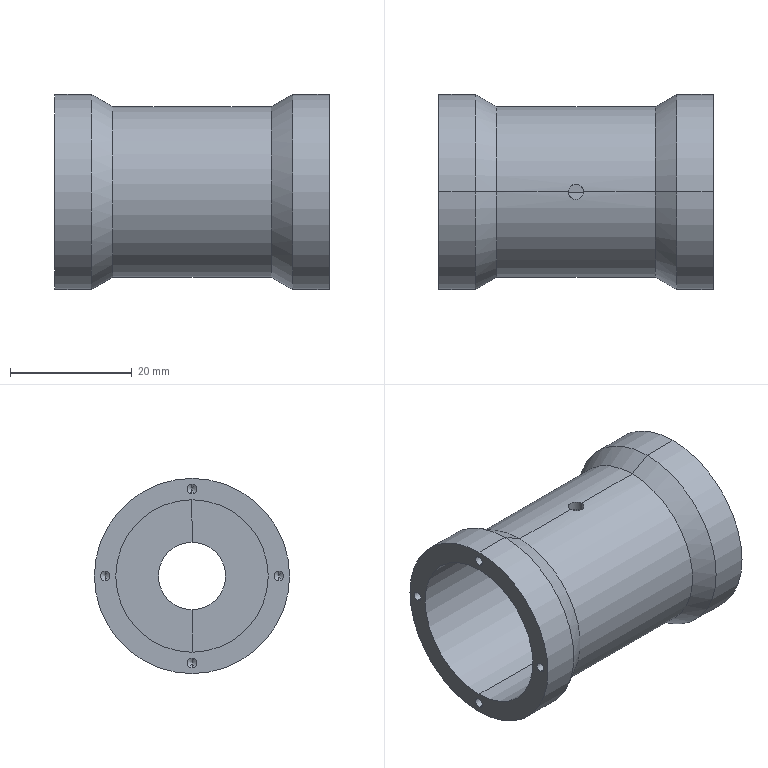Part | SolidWorks | features HoleWzd 2, ICE 1, Revolution 1 | 1 solid | 61 faces | box 45.002 x 32 x 32 mm | volume 10043 mm3 | cylinder 30 | cone 28 | plane 3 | commonest cylinder face diameters 1.6 x16 32 x4 2.5 x2 20.408 x2 24.608 x2 25 x2